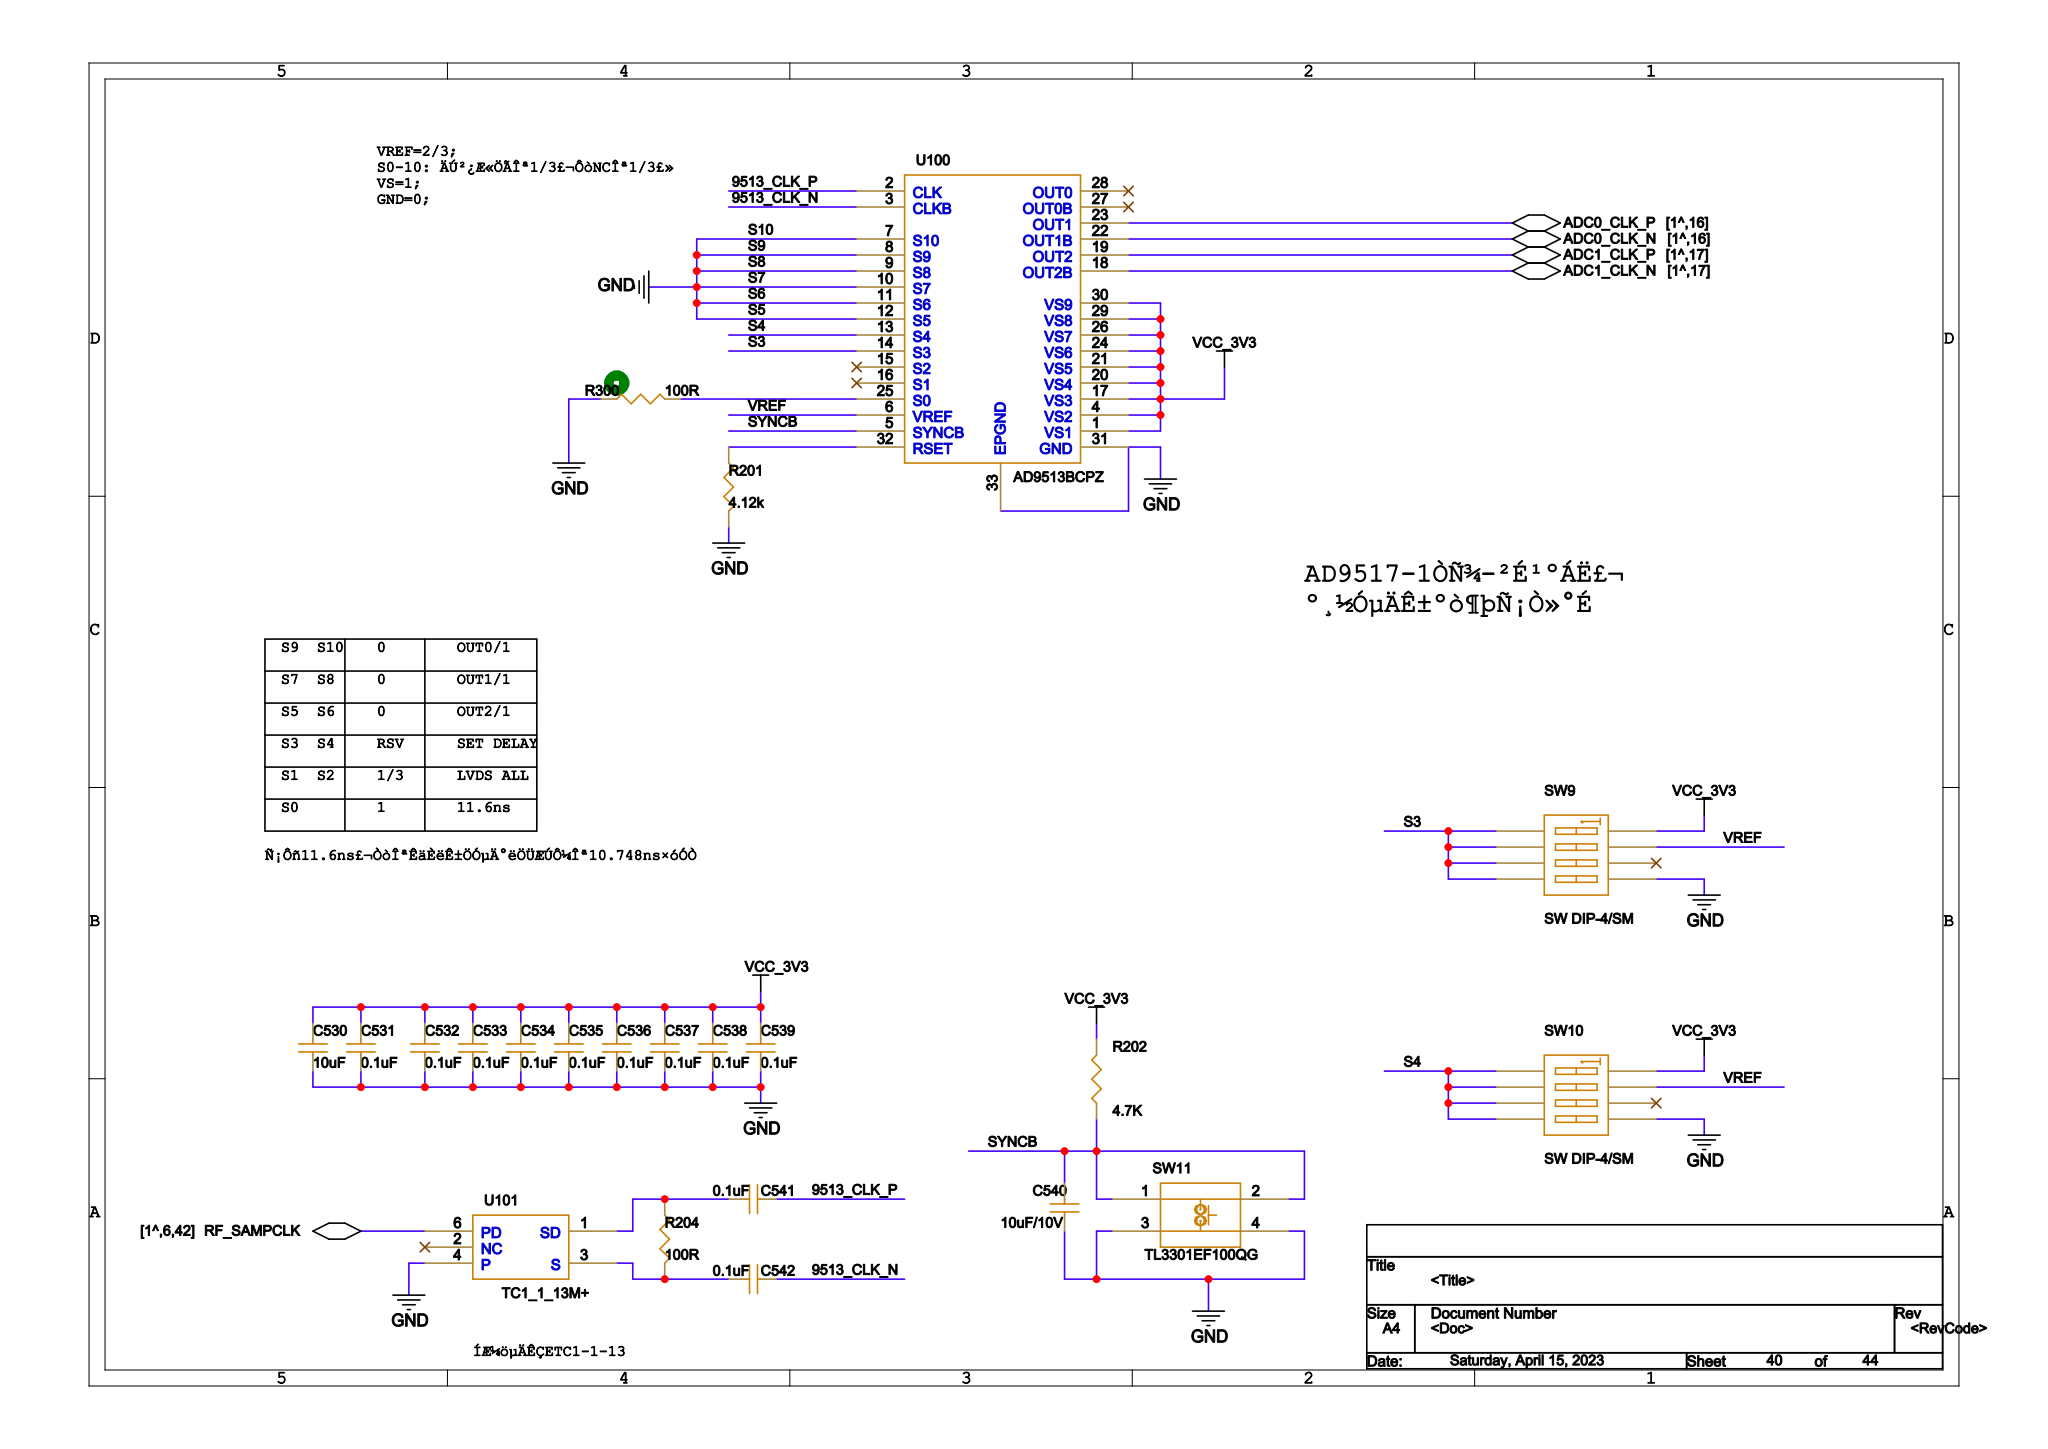Circuit board | Cadence Allegro | 1034 parts | 912 nets | one sheet of the schematic
Parts on this sheet (reference | value | footprint):
C530 | 10uF | C0402
C531 | 0.1uF | C0402
C532 | 0.1uF | C0402
C533 | 0.1uF | C0402
C534 | 0.1uF | C0402
C535 | 0.1uF | C0402
C536 | 0.1uF | C0402
C537 | 0.1uF | C0402
C538 | 0.1uF | C0402
C539 | 0.1uF | C0402
C540 | 10uF/10V | C0402
C541 | 0.1uF | C0402
C542 | 0.1uF | C0402
R201 | 4.12k | R0402
R202 | 4.7k | R0402
R204 | 100R | R0402
R300 | 100R | C0402
SW9 | SW DIP-4/SM | SW_4_SOP
SW10 | SW DIP-4/SM | SW_4_SOP
SW11 | TL3301EF100QG | GULLWING4
U100 | AD9513BCPZ | AD9513_LFCSP32
U101 | TC1_1_13M+ | TC1_1_13M_SMD
Nets of these parts (net: part-pin ...):
GND: C530-1 C531-1 C532-1 C533-1 C534-1 C535-1 C536-1 C537-1 C538-1 C539-1 C540-1 R201-2 R300-1 SW9-5 SW10-5 SW11-3 SW11-4 U101-4 U100-7 U100-8 U100-9 U100-10 U100-11 U100-12 U100-31 U100-33
VCC_3V3: C530-2 C531-2 C532-2 C533-2 C534-2 C535-2 C536-2 C537-2 C538-2 C539-2 R202-2 SW9-8 SW10-8 U100-1 U100-4 U100-17 U100-20 U100-21 U100-24 U100-26 U100-29 U100-30
N14593704: R300-2 U100-25
S4: SW10-1 SW10-2 SW10-3 SW10-4 U100-13
VREF: SW9-7 SW10-7 U100-6
S3: SW9-1 SW9-2 SW9-3 SW9-4 U100-14
9513_CLK_P: C541-1 U100-2
9513_CLK_N: C542-1 U100-3
N14137095: R201-1 U100-32
SYNCB: C540-2 R202-1 SW11-1 SW11-2 U100-5
N188110: U101-6
N14130954: C541-2 R204-1 U101-1
N14130946: C542-2 R204-2 U101-3